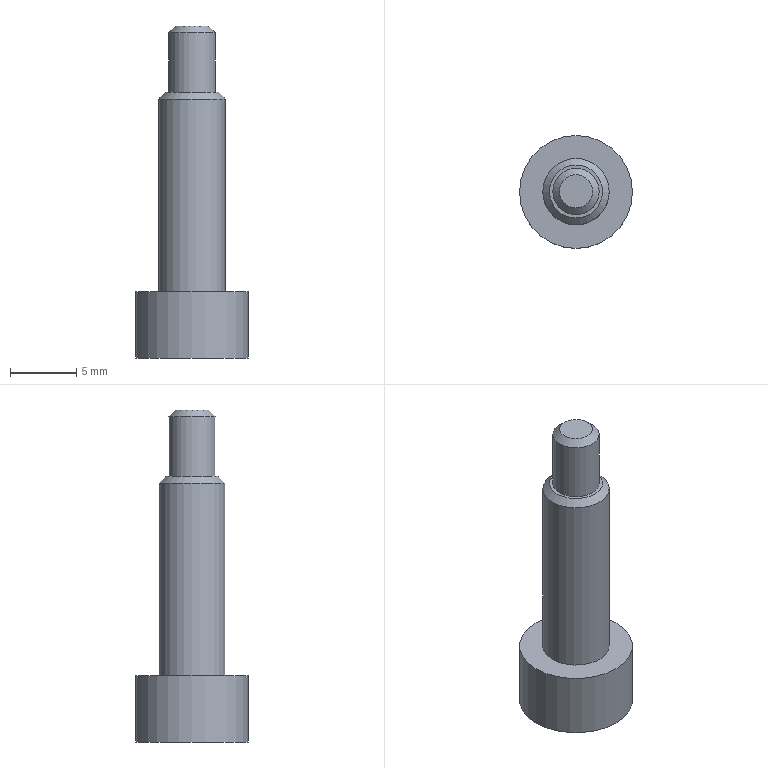Part | STEP file | 1 solid | 16 faces | box 8.5 x 8.5 x 25 mm | volume 577.553 mm3 | plane 11 | cylinder 3 | cone 2 | commonest cylinder face diameters 3.5 x1 5 x1 8.5 x1
STEP:
#1=CARTESIAN_POINT('',(0.,0.,0.));
#2=DIRECTION('',(0.,0.,1.));
#3=DIRECTION('',(1.,0.,0.));
#4=AXIS2_PLACEMENT_3D('',#1,#2,#3);
#5=CARTESIAN_POINT('',(1811.657,370.98,-34.906));
#6=VERTEX_POINT('',#5);
#7=CARTESIAN_POINT('',(1815.907,370.98,-34.906));
#8=DIRECTION('',(0.,0.,-1.));
#9=DIRECTION('',(-1.,0.,0.));
#10=AXIS2_PLACEMENT_3D('',#7,#8,#9);
#11=CIRCLE('',#10,4.25);
#12=CARTESIAN_POINT('',(1811.657,370.98,-34.906));
#13=DIRECTION('',(0.,0.,1.));
#14=DIRECTION('',(1.,0.,0.));
#15=AXIS2_PLACEMENT_3D('',#12,#13,#14);
#16=PLANE('',#15);
#17=CARTESIAN_POINT('',(0.,0.));
#18=CARTESIAN_POINT('',(0.,7.361));
#19=CARTESIAN_POINT('',(6.375,3.681));
#20=CARTESIAN_POINT('',(12.75,0.));
#21=CARTESIAN_POINT('',(6.375,-3.681));
#22=CARTESIAN_POINT('',(0.,-7.361));
#23=CARTESIAN_POINT('',(0.,0.));
#24=(BOUNDED_CURVE()B_SPLINE_CURVE(2,(#17,#18,#19,#20,#21,#22,#23),.UNSPECIFIED.,.T.,.F.)B_SPLINE_CURVE_WITH_KNOTS((1,2,2,2,2,1),(-2.094,0.,2.094,4.189,6.283,8.378),.UNSPECIFIED.)CURVE()GEOMETRIC_REPRESENTATION_ITEM()RATIONAL_B_SPLINE_CURVE((1.,0.5,1.,0.5,1.,0.5,1.))REPRESENTATION_ITEM(''));
#25=(GEOMETRIC_REPRESENTATION_CONTEXT(2)PARAMETRIC_REPRESENTATION_CONTEXT()REPRESENTATION_CONTEXT('',''));
#26=DEFINITIONAL_REPRESENTATION('',(#24),#25);
#27=PCURVE('',#16,#26);
#28=CARTESIAN_POINT('',(1815.907,370.98,1.494));
#29=DIRECTION('',(0.,0.,-1.));
#30=DIRECTION('',(-1.,0.,0.));
#31=AXIS2_PLACEMENT_3D('',#28,#29,#30);
#32=CYLINDRICAL_SURFACE('',#31,4.25);
#33=CARTESIAN_POINT('',(0.,36.4));
#34=DIRECTION('',(1.,0.));
#35=VECTOR('',#34,1.);
#36=LINE('',#33,#35);
#37=(GEOMETRIC_REPRESENTATION_CONTEXT(2)PARAMETRIC_REPRESENTATION_CONTEXT()REPRESENTATION_CONTEXT('',''));
#38=DEFINITIONAL_REPRESENTATION('',(#36),#37);
#39=PCURVE('',#32,#38);
#40=SURFACE_CURVE('',#11,(#27,#39),.PCURVE_S1.);
#41=EDGE_CURVE('',#6,#6,#40,.T.);
#42=ORIENTED_EDGE('',*,*,#41,.T.);
#43=EDGE_LOOP('',(#42));
#44=FACE_BOUND('',#43,.T.);
#45=CARTESIAN_POINT('',(1817.062,372.98,-34.906));
#46=VERTEX_POINT('',#45);
#47=CARTESIAN_POINT('',(1814.752,372.98,-34.906));
#48=VERTEX_POINT('',#47);
#49=CARTESIAN_POINT('',(1817.062,372.98,-34.906));
#50=DIRECTION('',(-1.,0.,0.));
#51=VECTOR('',#50,1.);
#52=LINE('',#49,#51);
#53=CARTESIAN_POINT('',(5.405,2.));
#54=DIRECTION('',(-1.,0.));
#55=VECTOR('',#54,1.);
#56=LINE('',#53,#55);
#57=(GEOMETRIC_REPRESENTATION_CONTEXT(2)PARAMETRIC_REPRESENTATION_CONTEXT()REPRESENTATION_CONTEXT('',''));
#58=DEFINITIONAL_REPRESENTATION('',(#56),#57);
#59=PCURVE('',#16,#58);
#60=CARTESIAN_POINT('',(1817.062,372.98,-31.606));
#61=DIRECTION('',(0.,-1.,0.));
#62=DIRECTION('',(-1.,0.,0.));
#63=AXIS2_PLACEMENT_3D('',#60,#61,#62);
#64=PLANE('',#63);
#65=CARTESIAN_POINT('',(0.,3.3));
#66=DIRECTION('',(1.,0.));
#67=VECTOR('',#66,1.);
#68=LINE('',#65,#67);
#69=(GEOMETRIC_REPRESENTATION_CONTEXT(2)PARAMETRIC_REPRESENTATION_CONTEXT()REPRESENTATION_CONTEXT('',''));
#70=DEFINITIONAL_REPRESENTATION('',(#68),#69);
#71=PCURVE('',#64,#70);
#72=SURFACE_CURVE('',#52,(#59,#71),.PCURVE_S1.);
#73=EDGE_CURVE('',#46,#48,#72,.T.);
#74=ORIENTED_EDGE('',*,*,#73,.T.);
#75=CARTESIAN_POINT('',(1813.598,370.98,-34.906));
#76=VERTEX_POINT('',#75);
#77=CARTESIAN_POINT('',(1814.752,372.98,-34.906));
#78=DIRECTION('',(-0.5,-0.866,0.));
#79=VECTOR('',#78,1.);
#80=LINE('',#77,#79);
#81=CARTESIAN_POINT('',(3.095,2.));
#82=DIRECTION('',(-0.5,-0.866));
#83=VECTOR('',#82,1.);
#84=LINE('',#81,#83);
#85=(GEOMETRIC_REPRESENTATION_CONTEXT(2)PARAMETRIC_REPRESENTATION_CONTEXT()REPRESENTATION_CONTEXT('',''));
#86=DEFINITIONAL_REPRESENTATION('',(#84),#85);
#87=PCURVE('',#16,#86);
#88=CARTESIAN_POINT('',(1814.752,372.98,-31.606));
#89=DIRECTION('',(0.866,-0.5,0.));
#90=DIRECTION('',(-0.5,-0.866,0.));
#91=AXIS2_PLACEMENT_3D('',#88,#89,#90);
#92=PLANE('',#91);
#93=CARTESIAN_POINT('',(0.,3.3));
#94=DIRECTION('',(1.,0.));
#95=VECTOR('',#94,1.);
#96=LINE('',#93,#95);
#97=(GEOMETRIC_REPRESENTATION_CONTEXT(2)PARAMETRIC_REPRESENTATION_CONTEXT()REPRESENTATION_CONTEXT('',''));
#98=DEFINITIONAL_REPRESENTATION('',(#96),#97);
#99=PCURVE('',#92,#98);
#100=SURFACE_CURVE('',#80,(#87,#99),.PCURVE_S1.);
#101=EDGE_CURVE('',#48,#76,#100,.T.);
#102=ORIENTED_EDGE('',*,*,#101,.T.);
#103=CARTESIAN_POINT('',(1814.752,368.98,-34.906));
#104=VERTEX_POINT('',#103);
#105=CARTESIAN_POINT('',(1813.598,370.98,-34.906));
#106=DIRECTION('',(0.5,-0.866,0.));
#107=VECTOR('',#106,1.);
#108=LINE('',#105,#107);
#109=CARTESIAN_POINT('',(1.941,0.));
#110=DIRECTION('',(0.5,-0.866));
#111=VECTOR('',#110,1.);
#112=LINE('',#109,#111);
#113=(GEOMETRIC_REPRESENTATION_CONTEXT(2)PARAMETRIC_REPRESENTATION_CONTEXT()REPRESENTATION_CONTEXT('',''));
#114=DEFINITIONAL_REPRESENTATION('',(#112),#113);
#115=PCURVE('',#16,#114);
#116=CARTESIAN_POINT('',(1813.598,370.98,-31.606));
#117=DIRECTION('',(0.866,0.5,0.));
#118=DIRECTION('',(0.5,-0.866,0.));
#119=AXIS2_PLACEMENT_3D('',#116,#117,#118);
#120=PLANE('',#119);
#121=CARTESIAN_POINT('',(0.,3.3));
#122=DIRECTION('',(1.,0.));
#123=VECTOR('',#122,1.);
#124=LINE('',#121,#123);
#125=(GEOMETRIC_REPRESENTATION_CONTEXT(2)PARAMETRIC_REPRESENTATION_CONTEXT()REPRESENTATION_CONTEXT('',''));
#126=DEFINITIONAL_REPRESENTATION('',(#124),#125);
#127=PCURVE('',#120,#126);
#128=SURFACE_CURVE('',#108,(#115,#127),.PCURVE_S1.);
#129=EDGE_CURVE('',#76,#104,#128,.T.);
#130=ORIENTED_EDGE('',*,*,#129,.T.);
#131=CARTESIAN_POINT('',(1817.062,368.98,-34.906));
#132=VERTEX_POINT('',#131);
#133=CARTESIAN_POINT('',(1814.752,368.98,-34.906));
#134=DIRECTION('',(1.,0.,0.));
#135=VECTOR('',#134,1.);
#136=LINE('',#133,#135);
#137=CARTESIAN_POINT('',(3.095,-2.));
#138=DIRECTION('',(1.,0.));
#139=VECTOR('',#138,1.);
#140=LINE('',#137,#139);
#141=(GEOMETRIC_REPRESENTATION_CONTEXT(2)PARAMETRIC_REPRESENTATION_CONTEXT()REPRESENTATION_CONTEXT('',''));
#142=DEFINITIONAL_REPRESENTATION('',(#140),#141);
#143=PCURVE('',#16,#142);
#144=CARTESIAN_POINT('',(1814.752,368.98,-31.606));
#145=DIRECTION('',(0.,1.,0.));
#146=DIRECTION('',(0.,0.,-1.));
#147=AXIS2_PLACEMENT_3D('',#144,#145,#146);
#148=PLANE('',#147);
#149=CARTESIAN_POINT('',(3.3,0.));
#150=DIRECTION('',(0.,-1.));
#151=VECTOR('',#150,1.);
#152=LINE('',#149,#151);
#153=(GEOMETRIC_REPRESENTATION_CONTEXT(2)PARAMETRIC_REPRESENTATION_CONTEXT()REPRESENTATION_CONTEXT('',''));
#154=DEFINITIONAL_REPRESENTATION('',(#152),#153);
#155=PCURVE('',#148,#154);
#156=SURFACE_CURVE('',#136,(#143,#155),.PCURVE_S1.);
#157=EDGE_CURVE('',#104,#132,#156,.T.);
#158=ORIENTED_EDGE('',*,*,#157,.T.);
#159=CARTESIAN_POINT('',(1818.217,370.98,-34.906));
#160=VERTEX_POINT('',#159);
#161=CARTESIAN_POINT('',(1817.062,368.98,-34.906));
#162=DIRECTION('',(0.5,0.866,0.));
#163=VECTOR('',#162,1.);
#164=LINE('',#161,#163);
#165=CARTESIAN_POINT('',(5.405,-2.));
#166=DIRECTION('',(0.5,0.866));
#167=VECTOR('',#166,1.);
#168=LINE('',#165,#167);
#169=(GEOMETRIC_REPRESENTATION_CONTEXT(2)PARAMETRIC_REPRESENTATION_CONTEXT()REPRESENTATION_CONTEXT('',''));
#170=DEFINITIONAL_REPRESENTATION('',(#168),#169);
#171=PCURVE('',#16,#170);
#172=CARTESIAN_POINT('',(1817.062,368.98,-31.606));
#173=DIRECTION('',(-0.866,0.5,0.));
#174=DIRECTION('',(0.5,0.866,0.));
#175=AXIS2_PLACEMENT_3D('',#172,#173,#174);
#176=PLANE('',#175);
#177=CARTESIAN_POINT('',(0.,3.3));
#178=DIRECTION('',(1.,0.));
#179=VECTOR('',#178,1.);
#180=LINE('',#177,#179);
#181=(GEOMETRIC_REPRESENTATION_CONTEXT(2)PARAMETRIC_REPRESENTATION_CONTEXT()REPRESENTATION_CONTEXT('',''));
#182=DEFINITIONAL_REPRESENTATION('',(#180),#181);
#183=PCURVE('',#176,#182);
#184=SURFACE_CURVE('',#164,(#171,#183),.PCURVE_S1.);
#185=EDGE_CURVE('',#132,#160,#184,.T.);
#186=ORIENTED_EDGE('',*,*,#185,.T.);
#187=CARTESIAN_POINT('',(1818.217,370.98,-34.906));
#188=DIRECTION('',(-0.5,0.866,0.));
#189=VECTOR('',#188,1.);
#190=LINE('',#187,#189);
#191=CARTESIAN_POINT('',(6.559,0.));
#192=DIRECTION('',(-0.5,0.866));
#193=VECTOR('',#192,1.);
#194=LINE('',#191,#193);
#195=(GEOMETRIC_REPRESENTATION_CONTEXT(2)PARAMETRIC_REPRESENTATION_CONTEXT()REPRESENTATION_CONTEXT('',''));
#196=DEFINITIONAL_REPRESENTATION('',(#194),#195);
#197=PCURVE('',#16,#196);
#198=CARTESIAN_POINT('',(1818.217,370.98,-31.606));
#199=DIRECTION('',(-0.866,-0.5,0.));
#200=DIRECTION('',(-0.5,0.866,0.));
#201=AXIS2_PLACEMENT_3D('',#198,#199,#200);
#202=PLANE('',#201);
#203=CARTESIAN_POINT('',(0.,3.3));
#204=DIRECTION('',(1.,0.));
#205=VECTOR('',#204,1.);
#206=LINE('',#203,#205);
#207=(GEOMETRIC_REPRESENTATION_CONTEXT(2)PARAMETRIC_REPRESENTATION_CONTEXT()REPRESENTATION_CONTEXT('',''));
#208=DEFINITIONAL_REPRESENTATION('',(#206),#207);
#209=PCURVE('',#202,#208);
#210=SURFACE_CURVE('',#190,(#197,#209),.PCURVE_S1.);
#211=EDGE_CURVE('',#160,#46,#210,.T.);
#212=ORIENTED_EDGE('',*,*,#211,.T.);
#213=EDGE_LOOP('',(#74,#102,#130,#158,#186,#212));
#214=FACE_BOUND('',#213,.T.);
#215=ADVANCED_FACE('',(#44,#214),#16,.F.);
#216=ORIENTED_EDGE('',*,*,#41,.F.);
#217=CARTESIAN_POINT('',(1811.657,370.98,-29.906));
#218=VERTEX_POINT('',#217);
#219=CARTESIAN_POINT('',(1811.657,370.98,-29.906));
#220=CARTESIAN_POINT('',(1811.657,370.98,-34.906));
#221=B_SPLINE_CURVE_WITH_KNOTS('',1,(#219,#220),.UNSPECIFIED.,.F.,.F.,(2,2),(31.4,36.4),.PIECEWISE_BEZIER_KNOTS.);
#222=CARTESIAN_POINT('',(0.,0.));
#223=DIRECTION('',(0.,1.));
#224=VECTOR('',#223,1.);
#225=LINE('',#222,#224);
#226=(GEOMETRIC_REPRESENTATION_CONTEXT(2)PARAMETRIC_REPRESENTATION_CONTEXT()REPRESENTATION_CONTEXT('',''));
#227=DEFINITIONAL_REPRESENTATION('',(#225),#226);
#228=PCURVE('',#32,#227);
#229=CARTESIAN_POINT('',(6.283,0.));
#230=DIRECTION('',(0.,1.));
#231=VECTOR('',#230,1.);
#232=LINE('',#229,#231);
#233=(GEOMETRIC_REPRESENTATION_CONTEXT(2)PARAMETRIC_REPRESENTATION_CONTEXT()REPRESENTATION_CONTEXT('',''));
#234=DEFINITIONAL_REPRESENTATION('',(#232),#233);
#235=PCURVE('',#32,#234);
#236=SEAM_CURVE('',#221,(#228,#235),.PCURVE_S1.);
#237=EDGE_CURVE('',#218,#6,#236,.T.);
#238=ORIENTED_EDGE('',*,*,#237,.F.);
#239=CARTESIAN_POINT('',(1815.907,370.98,-29.906));
#240=DIRECTION('',(0.,0.,-1.));
#241=DIRECTION('',(-1.,0.,0.));
#242=AXIS2_PLACEMENT_3D('',#239,#240,#241);
#243=CIRCLE('',#242,4.25);
#244=CARTESIAN_POINT('',(0.,31.4));
#245=DIRECTION('',(1.,0.));
#246=VECTOR('',#245,1.);
#247=LINE('',#244,#246);
#248=(GEOMETRIC_REPRESENTATION_CONTEXT(2)PARAMETRIC_REPRESENTATION_CONTEXT()REPRESENTATION_CONTEXT('',''));
#249=DEFINITIONAL_REPRESENTATION('',(#247),#248);
#250=PCURVE('',#32,#249);
#251=CARTESIAN_POINT('',(1813.407,370.98,-29.906));
#252=DIRECTION('',(0.,0.,-1.));
#253=DIRECTION('',(-1.,0.,0.));
#254=AXIS2_PLACEMENT_3D('',#251,#252,#253);
#255=PLANE('',#254);
#256=CARTESIAN_POINT('',(-2.5,0.));
#257=DIRECTION('',(1.,0.));
#258=AXIS2_PLACEMENT_2D('',#256,#257);
#259=CIRCLE('',#258,4.25);
#260=(GEOMETRIC_REPRESENTATION_CONTEXT(2)PARAMETRIC_REPRESENTATION_CONTEXT()REPRESENTATION_CONTEXT('',''));
#261=DEFINITIONAL_REPRESENTATION('',(#259),#260);
#262=PCURVE('',#255,#261);
#263=SURFACE_CURVE('',#243,(#250,#262),.PCURVE_S1.);
#264=EDGE_CURVE('',#218,#218,#263,.T.);
#265=ORIENTED_EDGE('',*,*,#264,.T.);
#266=ORIENTED_EDGE('',*,*,#237,.T.);
#267=EDGE_LOOP('',(#216,#238,#265,#266));
#268=FACE_BOUND('',#267,.T.);
#269=ADVANCED_FACE('',(#268),#32,.T.);
#270=ORIENTED_EDGE('',*,*,#264,.F.);
#271=EDGE_LOOP('',(#270));
#272=FACE_BOUND('',#271,.T.);
#273=CARTESIAN_POINT('',(1813.407,370.98,-29.906));
#274=VERTEX_POINT('',#273);
#275=CARTESIAN_POINT('',(1815.907,370.98,-29.906));
#276=DIRECTION('',(0.,0.,-1.));
#277=DIRECTION('',(-1.,0.,0.));
#278=AXIS2_PLACEMENT_3D('',#275,#276,#277);
#279=CIRCLE('',#278,2.5);
#280=CARTESIAN_POINT('',(-2.5,0.));
#281=DIRECTION('',(1.,0.));
#282=AXIS2_PLACEMENT_2D('',#280,#281);
#283=CIRCLE('',#282,2.5);
#284=(GEOMETRIC_REPRESENTATION_CONTEXT(2)PARAMETRIC_REPRESENTATION_CONTEXT()REPRESENTATION_CONTEXT('',''));
#285=DEFINITIONAL_REPRESENTATION('',(#283),#284);
#286=PCURVE('',#255,#285);
#287=CARTESIAN_POINT('',(1815.907,370.98,1.494));
#288=DIRECTION('',(0.,0.,-1.));
#289=DIRECTION('',(-1.,0.,0.));
#290=AXIS2_PLACEMENT_3D('',#287,#288,#289);
#291=CYLINDRICAL_SURFACE('',#290,2.5);
#292=CARTESIAN_POINT('',(0.,31.4));
#293=DIRECTION('',(1.,0.));
#294=VECTOR('',#293,1.);
#295=LINE('',#292,#294);
#296=(GEOMETRIC_REPRESENTATION_CONTEXT(2)PARAMETRIC_REPRESENTATION_CONTEXT()REPRESENTATION_CONTEXT('',''));
#297=DEFINITIONAL_REPRESENTATION('',(#295),#296);
#298=PCURVE('',#291,#297);
#299=SURFACE_CURVE('',#279,(#286,#298),.PCURVE_S1.);
#300=EDGE_CURVE('',#274,#274,#299,.T.);
#301=ORIENTED_EDGE('',*,*,#300,.T.);
#302=EDGE_LOOP('',(#301));
#303=FACE_BOUND('',#302,.T.);
#304=ADVANCED_FACE('',(#272,#303),#255,.F.);
#305=CARTESIAN_POINT('',(1818.407,370.98,-15.406));
#306=VERTEX_POINT('',#305);
#307=CARTESIAN_POINT('',(1813.407,370.98,-15.406));
#308=VERTEX_POINT('',#307);
#309=CARTESIAN_POINT('',(1815.907,370.98,-15.406));
#310=DIRECTION('',(0.,0.,-1.));
#311=DIRECTION('',(1.,0.,0.));
#312=AXIS2_PLACEMENT_3D('',#309,#310,#311);
#313=CIRCLE('',#312,2.5);
#314=CARTESIAN_POINT('',(3.142,16.9));
#315=DIRECTION('',(1.,0.));
#316=VECTOR('',#315,1.);
#317=LINE('',#314,#316);
#318=(GEOMETRIC_REPRESENTATION_CONTEXT(2)PARAMETRIC_REPRESENTATION_CONTEXT()REPRESENTATION_CONTEXT('',''));
#319=DEFINITIONAL_REPRESENTATION('',(#317),#318);
#320=PCURVE('',#291,#319);
#321=CARTESIAN_POINT('',(1815.907,370.98,-15.406));
#322=DIRECTION('',(0.,0.,-1.));
#323=DIRECTION('',(-1.,0.,0.));
#324=AXIS2_PLACEMENT_3D('',#321,#322,#323);
#325=CONICAL_SURFACE('',#324,2.5,0.7854);
#326=CARTESIAN_POINT('',(3.142,0.));
#327=DIRECTION('',(1.,0.));
#328=VECTOR('',#327,1.);
#329=LINE('',#326,#328);
#330=(GEOMETRIC_REPRESENTATION_CONTEXT(2)PARAMETRIC_REPRESENTATION_CONTEXT()REPRESENTATION_CONTEXT('',''));
#331=DEFINITIONAL_REPRESENTATION('',(#329),#330);
#332=PCURVE('',#325,#331);
#333=SURFACE_CURVE('',#313,(#320,#332),.PCURVE_S1.);
#334=EDGE_CURVE('',#306,#308,#333,.T.);
#335=ORIENTED_EDGE('',*,*,#334,.T.);
#336=CARTESIAN_POINT('',(1813.407,370.98,-15.406));
#337=CARTESIAN_POINT('',(1813.407,370.98,-29.906));
#338=B_SPLINE_CURVE_WITH_KNOTS('',1,(#336,#337),.UNSPECIFIED.,.F.,.F.,(2,2),(16.9,31.4),.PIECEWISE_BEZIER_KNOTS.);
#339=CARTESIAN_POINT('',(6.283,0.));
#340=DIRECTION('',(0.,1.));
#341=VECTOR('',#340,1.);
#342=LINE('',#339,#341);
#343=(GEOMETRIC_REPRESENTATION_CONTEXT(2)PARAMETRIC_REPRESENTATION_CONTEXT()REPRESENTATION_CONTEXT('',''));
#344=DEFINITIONAL_REPRESENTATION('',(#342),#343);
#345=PCURVE('',#291,#344);
#346=CARTESIAN_POINT('',(0.,0.));
#347=DIRECTION('',(0.,1.));
#348=VECTOR('',#347,1.);
#349=LINE('',#346,#348);
#350=(GEOMETRIC_REPRESENTATION_CONTEXT(2)PARAMETRIC_REPRESENTATION_CONTEXT()REPRESENTATION_CONTEXT('',''));
#351=DEFINITIONAL_REPRESENTATION('',(#349),#350);
#352=PCURVE('',#291,#351);
#353=SEAM_CURVE('',#338,(#345,#352),.PCURVE_S1.);
#354=EDGE_CURVE('',#308,#274,#353,.T.);
#355=ORIENTED_EDGE('',*,*,#354,.T.);
#356=ORIENTED_EDGE('',*,*,#300,.F.);
#357=ORIENTED_EDGE('',*,*,#354,.F.);
#358=CARTESIAN_POINT('',(1815.907,370.98,-15.406));
#359=DIRECTION('',(0.,0.,-1.));
#360=DIRECTION('',(1.,0.,0.));
#361=AXIS2_PLACEMENT_3D('',#358,#359,#360);
#362=CIRCLE('',#361,2.5);
#363=CARTESIAN_POINT('',(-3.142,16.9));
#364=DIRECTION('',(1.,0.));
#365=VECTOR('',#364,1.);
#366=LINE('',#363,#365);
#367=(GEOMETRIC_REPRESENTATION_CONTEXT(2)PARAMETRIC_REPRESENTATION_CONTEXT()REPRESENTATION_CONTEXT('',''));
#368=DEFINITIONAL_REPRESENTATION('',(#366),#367);
#369=PCURVE('',#291,#368);
#370=CARTESIAN_POINT('',(3.142,0.));
#371=DIRECTION('',(1.,0.));
#372=VECTOR('',#371,1.);
#373=LINE('',#370,#372);
#374=(GEOMETRIC_REPRESENTATION_CONTEXT(2)PARAMETRIC_REPRESENTATION_CONTEXT()REPRESENTATION_CONTEXT('',''));
#375=DEFINITIONAL_REPRESENTATION('',(#373),#374);
#376=PCURVE('',#325,#375);
#377=SURFACE_CURVE('',#362,(#369,#376),.PCURVE_S1.);
#378=EDGE_CURVE('',#308,#306,#377,.T.);
#379=ORIENTED_EDGE('',*,*,#378,.T.);
#380=EDGE_LOOP('',(#335,#355,#356,#357,#379));
#381=FACE_BOUND('',#380,.T.);
#382=ADVANCED_FACE('',(#381),#291,.T.);
#383=ORIENTED_EDGE('',*,*,#73,.F.);
#384=CARTESIAN_POINT('',(1817.062,372.98,-31.606));
#385=VERTEX_POINT('',#384);
#386=CARTESIAN_POINT('',(1817.062,372.98,-31.606));
#387=DIRECTION('',(0.,0.,1.));
#388=VECTOR('',#387,1.);
#389=LINE('',#386,#388);
#390=CARTESIAN_POINT('',(0.,0.));
#391=DIRECTION('',(0.,-1.));
#392=VECTOR('',#391,1.);
#393=LINE('',#390,#392);
#394=(GEOMETRIC_REPRESENTATION_CONTEXT(2)PARAMETRIC_REPRESENTATION_CONTEXT()REPRESENTATION_CONTEXT('',''));
#395=DEFINITIONAL_REPRESENTATION('',(#393),#394);
#396=PCURVE('',#64,#395);
#397=CARTESIAN_POINT('',(2.309,0.));
#398=DIRECTION('',(0.,-1.));
#399=VECTOR('',#398,1.);
#400=LINE('',#397,#399);
#401=(GEOMETRIC_REPRESENTATION_CONTEXT(2)PARAMETRIC_REPRESENTATION_CONTEXT()REPRESENTATION_CONTEXT('',''));
#402=DEFINITIONAL_REPRESENTATION('',(#400),#401);
#403=PCURVE('',#202,#402);
#404=SURFACE_CURVE('',#389,(#396,#403),.PCURVE_S1.);
#405=EDGE_CURVE('',#46,#385,#404,.T.);
#406=ORIENTED_EDGE('',*,*,#405,.T.);
#407=CARTESIAN_POINT('',(1814.752,372.98,-31.606));
#408=VERTEX_POINT('',#407);
#409=CARTESIAN_POINT('',(1817.062,372.98,-31.606));
#410=DIRECTION('',(1.,0.,0.));
#411=VECTOR('',#410,1.);
#412=LINE('',#409,#411);
#413=CARTESIAN_POINT('',(0.,0.));
#414=DIRECTION('',(-1.,0.));
#415=VECTOR('',#414,1.);
#416=LINE('',#413,#415);
#417=(GEOMETRIC_REPRESENTATION_CONTEXT(2)PARAMETRIC_REPRESENTATION_CONTEXT()REPRESENTATION_CONTEXT('',''));
#418=DEFINITIONAL_REPRESENTATION('',(#416),#417);
#419=PCURVE('',#64,#418);
#420=CARTESIAN_POINT('',(1815.907,370.98,-31.606));
#421=DIRECTION('',(0.,0.,1.));
#422=DIRECTION('',(1.,0.,0.));
#423=AXIS2_PLACEMENT_3D('',#420,#421,#422);
#424=PLANE('',#423);
#425=CARTESIAN_POINT('',(1.155,2.));
#426=DIRECTION('',(1.,0.));
#427=VECTOR('',#426,1.);
#428=LINE('',#425,#427);
#429=(GEOMETRIC_REPRESENTATION_CONTEXT(2)PARAMETRIC_REPRESENTATION_CONTEXT()REPRESENTATION_CONTEXT('',''));
#430=DEFINITIONAL_REPRESENTATION('',(#428),#429);
#431=PCURVE('',#424,#430);
#432=SURFACE_CURVE('',#412,(#419,#431),.PCURVE_S1.);
#433=EDGE_CURVE('',#408,#385,#432,.T.);
#434=ORIENTED_EDGE('',*,*,#433,.F.);
#435=CARTESIAN_POINT('',(1814.752,372.98,-31.606));
#436=DIRECTION('',(0.,0.,1.));
#437=VECTOR('',#436,1.);
#438=LINE('',#435,#437);
#439=CARTESIAN_POINT('',(2.309,0.));
#440=DIRECTION('',(0.,-1.));
#441=VECTOR('',#440,1.);
#442=LINE('',#439,#441);
#443=(GEOMETRIC_REPRESENTATION_CONTEXT(2)PARAMETRIC_REPRESENTATION_CONTEXT()REPRESENTATION_CONTEXT('',''));
#444=DEFINITIONAL_REPRESENTATION('',(#442),#443);
#445=PCURVE('',#64,#444);
#446=CARTESIAN_POINT('',(0.,0.));
#447=DIRECTION('',(0.,-1.));
#448=VECTOR('',#447,1.);
#449=LINE('',#446,#448);
#450=(GEOMETRIC_REPRESENTATION_CONTEXT(2)PARAMETRIC_REPRESENTATION_CONTEXT()REPRESENTATION_CONTEXT('',''));
#451=DEFINITIONAL_REPRESENTATION('',(#449),#450);
#452=PCURVE('',#92,#451);
#453=SURFACE_CURVE('',#438,(#445,#452),.PCURVE_S1.);
#454=EDGE_CURVE('',#48,#408,#453,.T.);
#455=ORIENTED_EDGE('',*,*,#454,.F.);
#456=EDGE_LOOP('',(#383,#406,#434,#455));
#457=FACE_BOUND('',#456,.T.);
#458=ADVANCED_FACE('',(#457),#64,.T.);
#459=ORIENTED_EDGE('',*,*,#101,.F.);
#460=ORIENTED_EDGE('',*,*,#454,.T.);
#461=CARTESIAN_POINT('',(1813.598,370.98,-31.606));
#462=VERTEX_POINT('',#461);
#463=CARTESIAN_POINT('',(1814.752,372.98,-31.606));
#464=DIRECTION('',(0.5,0.866,0.));
#465=VECTOR('',#464,1.);
#466=LINE('',#463,#465);
#467=CARTESIAN_POINT('',(0.,0.));
#468=DIRECTION('',(-1.,0.));
#469=VECTOR('',#468,1.);
#470=LINE('',#467,#469);
#471=(GEOMETRIC_REPRESENTATION_CONTEXT(2)PARAMETRIC_REPRESENTATION_CONTEXT()REPRESENTATION_CONTEXT('',''));
#472=DEFINITIONAL_REPRESENTATION('',(#470),#471);
#473=PCURVE('',#92,#472);
#474=CARTESIAN_POINT('',(-1.155,2.));
#475=DIRECTION('',(0.5,0.866));
#476=VECTOR('',#475,1.);
#477=LINE('',#474,#476);
#478=(GEOMETRIC_REPRESENTATION_CONTEXT(2)PARAMETRIC_REPRESENTATION_CONTEXT()REPRESENTATION_CONTEXT('',''));
#479=DEFINITIONAL_REPRESENTATION('',(#477),#478);
#480=PCURVE('',#424,#479);
#481=SURFACE_CURVE('',#466,(#473,#480),.PCURVE_S1.);
#482=EDGE_CURVE('',#462,#408,#481,.T.);
#483=ORIENTED_EDGE('',*,*,#482,.F.);
#484=CARTESIAN_POINT('',(1813.598,370.98,-31.606));
#485=DIRECTION('',(0.,0.,1.));
#486=VECTOR('',#485,1.);
#487=LINE('',#484,#486);
#488=CARTESIAN_POINT('',(2.309,0.));
#489=DIRECTION('',(0.,-1.));
#490=VECTOR('',#489,1.);
#491=LINE('',#488,#490);
#492=(GEOMETRIC_REPRESENTATION_CONTEXT(2)PARAMETRIC_REPRESENTATION_CONTEXT()REPRESENTATION_CONTEXT('',''));
#493=DEFINITIONAL_REPRESENTATION('',(#491),#492);
#494=PCURVE('',#92,#493);
#495=CARTESIAN_POINT('',(0.,0.));
#496=DIRECTION('',(0.,-1.));
#497=VECTOR('',#496,1.);
#498=LINE('',#495,#497);
#499=(GEOMETRIC_REPRESENTATION_CONTEXT(2)PARAMETRIC_REPRESENTATION_CONTEXT()REPRESENTATION_CONTEXT('',''));
#500=DEFINITIONAL_REPRESENTATION('',(#498),#499);
#501=PCURVE('',#120,#500);
#502=SURFACE_CURVE('',#487,(#494,#501),.PCURVE_S1.);
#503=EDGE_CURVE('',#76,#462,#502,.T.);
#504=ORIENTED_EDGE('',*,*,#503,.F.);
#505=EDGE_LOOP('',(#459,#460,#483,#504));
#506=FACE_BOUND('',#505,.T.);
#507=ADVANCED_FACE('',(#506),#92,.T.);
#508=ORIENTED_EDGE('',*,*,#129,.F.);
#509=ORIENTED_EDGE('',*,*,#503,.T.);
#510=CARTESIAN_POINT('',(1814.752,368.98,-31.606));
#511=VERTEX_POINT('',#510);
#512=CARTESIAN_POINT('',(1813.598,370.98,-31.606));
#513=DIRECTION('',(-0.5,0.866,0.));
#514=VECTOR('',#513,1.);
#515=LINE('',#512,#514);
#516=CARTESIAN_POINT('',(0.,0.));
#517=DIRECTION('',(-1.,0.));
#518=VECTOR('',#517,1.);
#519=LINE('',#516,#518);
#520=(GEOMETRIC_REPRESENTATION_CONTEXT(2)PARAMETRIC_REPRESENTATION_CONTEXT()REPRESENTATION_CONTEXT('',''));
#521=DEFINITIONAL_REPRESENTATION('',(#519),#520);
#522=PCURVE('',#120,#521);
#523=CARTESIAN_POINT('',(-2.309,0.));
#524=DIRECTION('',(-0.5,0.866));
#525=VECTOR('',#524,1.);
#526=LINE('',#523,#525);
#527=(GEOMETRIC_REPRESENTATION_CONTEXT(2)PARAMETRIC_REPRESENTATION_CONTEXT()REPRESENTATION_CONTEXT('',''));
#528=DEFINITIONAL_REPRESENTATION('',(#526),#527);
#529=PCURVE('',#424,#528);
#530=SURFACE_CURVE('',#515,(#522,#529),.PCURVE_S1.);
#531=EDGE_CURVE('',#511,#462,#530,.T.);
#532=ORIENTED_EDGE('',*,*,#531,.F.);
#533=CARTESIAN_POINT('',(1814.752,368.98,-31.606));
#534=DIRECTION('',(0.,0.,1.));
#535=VECTOR('',#534,1.);
#536=LINE('',#533,#535);
#537=CARTESIAN_POINT('',(2.309,0.));
#538=DIRECTION('',(0.,-1.));
#539=VECTOR('',#538,1.);
#540=LINE('',#537,#539);
#541=(GEOMETRIC_REPRESENTATION_CONTEXT(2)PARAMETRIC_REPRESENTATION_CONTEXT()REPRESENTATION_CONTEXT('',''));
#542=DEFINITIONAL_REPRESENTATION('',(#540),#541);
#543=PCURVE('',#120,#542);
#544=CARTESIAN_POINT('',(0.,0.));
#545=DIRECTION('',(-1.,0.));
#546=VECTOR('',#545,1.);
#547=LINE('',#544,#546);
#548=(GEOMETRIC_REPRESENTATION_CONTEXT(2)PARAMETRIC_REPRESENTATION_CONTEXT()REPRESENTATION_CONTEXT('',''));
#549=DEFINITIONAL_REPRESENTATION('',(#547),#548);
#550=PCURVE('',#148,#549);
#551=SURFACE_CURVE('',#536,(#543,#550),.PCURVE_S1.);
#552=EDGE_CURVE('',#104,#511,#551,.T.);
#553=ORIENTED_EDGE('',*,*,#552,.F.);
#554=EDGE_LOOP('',(#508,#509,#532,#553));
#555=FACE_BOUND('',#554,.T.);
#556=ADVANCED_FACE('',(#555),#120,.T.);
#557=ORIENTED_EDGE('',*,*,#157,.F.);
#558=ORIENTED_EDGE('',*,*,#552,.T.);
#559=CARTESIAN_POINT('',(1817.062,368.98,-31.606));
#560=VERTEX_POINT('',#559);
#561=CARTESIAN_POINT('',(1814.752,368.98,-31.606));
#562=DIRECTION('',(-1.,0.,0.));
#563=VECTOR('',#562,1.);
#564=LINE('',#561,#563);
#565=CARTESIAN_POINT('',(0.,0.));
#566=DIRECTION('',(0.,1.));
#567=VECTOR('',#566,1.);
#568=LINE('',#565,#567);
#569=(GEOMETRIC_REPRESENTATION_CONTEXT(2)PARAMETRIC_REPRESENTATION_CONTEXT()REPRESENTATION_CONTEXT('',''));
#570=DEFINITIONAL_REPRESENTATION('',(#568),#569);
#571=PCURVE('',#148,#570);
#572=CARTESIAN_POINT('',(-1.155,-2.));
#573=DIRECTION('',(-1.,0.));
#574=VECTOR('',#573,1.);
#575=LINE('',#572,#574);
#576=(GEOMETRIC_REPRESENTATION_CONTEXT(2)PARAMETRIC_REPRESENTATION_CONTEXT()REPRESENTATION_CONTEXT('',''));
#577=DEFINITIONAL_REPRESENTATION('',(#575),#576);
#578=PCURVE('',#424,#577);
#579=SURFACE_CURVE('',#564,(#571,#578),.PCURVE_S1.);
#580=EDGE_CURVE('',#560,#511,#579,.T.);
#581=ORIENTED_EDGE('',*,*,#580,.F.);
#582=CARTESIAN_POINT('',(1817.062,368.98,-31.606));
#583=DIRECTION('',(0.,0.,1.));
#584=VECTOR('',#583,1.);
#585=LINE('',#582,#584);
#586=CARTESIAN_POINT('',(0.,-2.309));
#587=DIRECTION('',(-1.,0.));
#588=VECTOR('',#587,1.);
#589=LINE('',#586,#588);
#590=(GEOMETRIC_REPRESENTATION_CONTEXT(2)PARAMETRIC_REPRESENTATION_CONTEXT()REPRESENTATION_CONTEXT('',''));
#591=DEFINITIONAL_REPRESENTATION('',(#589),#590);
#592=PCURVE('',#148,#591);
#593=CARTESIAN_POINT('',(0.,0.));
#594=DIRECTION('',(0.,-1.));
#595=VECTOR('',#594,1.);
#596=LINE('',#593,#595);
#597=(GEOMETRIC_REPRESENTATION_CONTEXT(2)PARAMETRIC_REPRESENTATION_CONTEXT()REPRESENTATION_CONTEXT('',''));
#598=DEFINITIONAL_REPRESENTATION('',(#596),#597);
#599=PCURVE('',#176,#598);
#600=SURFACE_CURVE('',#585,(#592,#599),.PCURVE_S1.);
#601=EDGE_CURVE('',#132,#560,#600,.T.);
#602=ORIENTED_EDGE('',*,*,#601,.F.);
#603=EDGE_LOOP('',(#557,#558,#581,#602));
#604=FACE_BOUND('',#603,.T.);
#605=ADVANCED_FACE('',(#604),#148,.T.);
#606=ORIENTED_EDGE('',*,*,#185,.F.);
#607=ORIENTED_EDGE('',*,*,#601,.T.);
#608=CARTESIAN_POINT('',(1818.217,370.98,-31.606));
#609=VERTEX_POINT('',#608);
#610=CARTESIAN_POINT('',(1817.062,368.98,-31.606));
#611=DIRECTION('',(-0.5,-0.866,0.));
#612=VECTOR('',#611,1.);
#613=LINE('',#610,#612);
#614=CARTESIAN_POINT('',(0.,0.));
#615=DIRECTION('',(-1.,0.));
#616=VECTOR('',#615,1.);
#617=LINE('',#614,#616);
#618=(GEOMETRIC_REPRESENTATION_CONTEXT(2)PARAMETRIC_REPRESENTATION_CONTEXT()REPRESENTATION_CONTEXT('',''));
#619=DEFINITIONAL_REPRESENTATION('',(#617),#618);
#620=PCURVE('',#176,#619);
#621=CARTESIAN_POINT('',(1.155,-2.));
#622=DIRECTION('',(-0.5,-0.866));
#623=VECTOR('',#622,1.);
#624=LINE('',#621,#623);
#625=(GEOMETRIC_REPRESENTATION_CONTEXT(2)PARAMETRIC_REPRESENTATION_CONTEXT()REPRESENTATION_CONTEXT('',''));
#626=DEFINITIONAL_REPRESENTATION('',(#624),#625);
#627=PCURVE('',#424,#626);
#628=SURFACE_CURVE('',#613,(#620,#627),.PCURVE_S1.);
#629=EDGE_CURVE('',#609,#560,#628,.T.);
#630=ORIENTED_EDGE('',*,*,#629,.F.);
#631=CARTESIAN_POINT('',(1818.217,370.98,-31.606));
#632=DIRECTION('',(0.,0.,1.));
#633=VECTOR('',#632,1.);
#634=LINE('',#631,#633);
#635=CARTESIAN_POINT('',(2.309,0.));
#636=DIRECTION('',(0.,-1.));
#637=VECTOR('',#636,1.);
#638=LINE('',#635,#637);
#639=(GEOMETRIC_REPRESENTATION_CONTEXT(2)PARAMETRIC_REPRESENTATION_CONTEXT()REPRESENTATION_CONTEXT('',''));
#640=DEFINITIONAL_REPRESENTATION('',(#638),#639);
#641=PCURVE('',#176,#640);
#642=CARTESIAN_POINT('',(0.,0.));
#643=DIRECTION('',(0.,-1.));
#644=VECTOR('',#643,1.);
#645=LINE('',#642,#644);
#646=(GEOMETRIC_REPRESENTATION_CONTEXT(2)PARAMETRIC_REPRESENTATION_CONTEXT()REPRESENTATION_CONTEXT('',''));
#647=DEFINITIONAL_REPRESENTATION('',(#645),#646);
#648=PCURVE('',#202,#647);
#649=SURFACE_CURVE('',#634,(#641,#648),.PCURVE_S1.);
#650=EDGE_CURVE('',#160,#609,#649,.T.);
#651=ORIENTED_EDGE('',*,*,#650,.F.);
#652=EDGE_LOOP('',(#606,#607,#630,#651));
#653=FACE_BOUND('',#652,.T.);
#654=ADVANCED_FACE('',(#653),#176,.T.);
#655=ORIENTED_EDGE('',*,*,#211,.F.);
#656=ORIENTED_EDGE('',*,*,#650,.T.);
#657=CARTESIAN_POINT('',(1818.217,370.98,-31.606));
#658=DIRECTION('',(0.5,-0.866,0.));
#659=VECTOR('',#658,1.);
#660=LINE('',#657,#659);
#661=CARTESIAN_POINT('',(0.,0.));
#662=DIRECTION('',(-1.,0.));
#663=VECTOR('',#662,1.);
#664=LINE('',#661,#663);
#665=(GEOMETRIC_REPRESENTATION_CONTEXT(2)PARAMETRIC_REPRESENTATION_CONTEXT()REPRESENTATION_CONTEXT('',''));
#666=DEFINITIONAL_REPRESENTATION('',(#664),#665);
#667=PCURVE('',#202,#666);
#668=CARTESIAN_POINT('',(2.309,0.));
#669=DIRECTION('',(0.5,-0.866));
#670=VECTOR('',#669,1.);
#671=LINE('',#668,#670);
#672=(GEOMETRIC_REPRESENTATION_CONTEXT(2)PARAMETRIC_REPRESENTATION_CONTEXT()REPRESENTATION_CONTEXT('',''));
#673=DEFINITIONAL_REPRESENTATION('',(#671),#672);
#674=PCURVE('',#424,#673);
#675=SURFACE_CURVE('',#660,(#667,#674),.PCURVE_S1.);
#676=EDGE_CURVE('',#385,#609,#675,.T.);
#677=ORIENTED_EDGE('',*,*,#676,.F.);
#678=ORIENTED_EDGE('',*,*,#405,.F.);
#679=EDGE_LOOP('',(#655,#656,#677,#678));
#680=FACE_BOUND('',#679,.T.);
#681=ADVANCED_FACE('',(#680),#202,.T.);
#682=ORIENTED_EDGE('',*,*,#433,.T.);
#683=ORIENTED_EDGE('',*,*,#676,.T.);
#684=ORIENTED_EDGE('',*,*,#629,.T.);
#685=ORIENTED_EDGE('',*,*,#580,.T.);
#686=ORIENTED_EDGE('',*,*,#531,.T.);
#687=ORIENTED_EDGE('',*,*,#482,.T.);
#688=EDGE_LOOP('',(#682,#683,#684,#685,#686,#687));
#689=FACE_BOUND('',#688,.T.);
#690=ADVANCED_FACE('',(#689),#424,.F.);
#691=CARTESIAN_POINT('',(1817.907,370.98,-14.906));
#692=VERTEX_POINT('',#691);
#693=CARTESIAN_POINT('',(1815.907,370.98,-14.906));
#694=DIRECTION('',(0.,0.,1.));
#695=DIRECTION('',(1.,0.,0.));
#696=AXIS2_PLACEMENT_3D('',#693,#694,#695);
#697=CIRCLE('',#696,2.);
#698=CARTESIAN_POINT('',(1815.907,370.98,-14.906));
#699=DIRECTION('',(0.,0.,1.));
#700=DIRECTION('',(1.,0.,0.));
#701=AXIS2_PLACEMENT_3D('',#698,#699,#700);
#702=PLANE('',#701);
#703=CARTESIAN_POINT('',(0.,0.));
#704=DIRECTION('',(1.,0.));
#705=AXIS2_PLACEMENT_2D('',#703,#704);
#706=CIRCLE('',#705,2.);
#707=(GEOMETRIC_REPRESENTATION_CONTEXT(2)PARAMETRIC_REPRESENTATION_CONTEXT()REPRESENTATION_CONTEXT('',''));
#708=DEFINITIONAL_REPRESENTATION('',(#706),#707);
#709=PCURVE('',#702,#708);
#710=CARTESIAN_POINT('',(9.425,-0.5));
#711=DIRECTION('',(-1.,0.));
#712=VECTOR('',#711,1.);
#713=LINE('',#710,#712);
#714=(GEOMETRIC_REPRESENTATION_CONTEXT(2)PARAMETRIC_REPRESENTATION_CONTEXT()REPRESENTATION_CONTEXT('',''));
#715=DEFINITIONAL_REPRESENTATION('',(#713),#714);
#716=PCURVE('',#325,#715);
#717=SURFACE_CURVE('',#697,(#709,#716),.PCURVE_S1.);
#718=EDGE_CURVE('',#692,#692,#717,.T.);
#719=ORIENTED_EDGE('',*,*,#718,.T.);
#720=EDGE_LOOP('',(#719));
#721=FACE_BOUND('',#720,.T.);
#722=CARTESIAN_POINT('',(1817.657,370.98,-14.906));
#723=VERTEX_POINT('',#722);
#724=CARTESIAN_POINT('',(1814.157,370.98,-14.906));
#725=VERTEX_POINT('',#724);
#726=CARTESIAN_POINT('',(1815.907,370.98,-14.906));
#727=DIRECTION('',(0.,0.,1.));
#728=DIRECTION('',(1.,0.,0.));
#729=AXIS2_PLACEMENT_3D('',#726,#727,#728);
#730=CIRCLE('',#729,1.75);
#731=CARTESIAN_POINT('',(0.,0.));
#732=DIRECTION('',(1.,0.));
#733=AXIS2_PLACEMENT_2D('',#731,#732);
#734=CIRCLE('',#733,1.75);
#735=(GEOMETRIC_REPRESENTATION_CONTEXT(2)PARAMETRIC_REPRESENTATION_CONTEXT()REPRESENTATION_CONTEXT('',''));
#736=DEFINITIONAL_REPRESENTATION('',(#734),#735);
#737=PCURVE('',#702,#736);
#738=CARTESIAN_POINT('',(1815.907,370.98,-9.906));
#739=DIRECTION('',(0.,0.,-1.));
#740=DIRECTION('',(-1.,0.,0.));
#741=AXIS2_PLACEMENT_3D('',#738,#739,#740);
#742=CYLINDRICAL_SURFACE('',#741,1.75);
#743=CARTESIAN_POINT('',(3.142,5.));
#744=DIRECTION('',(-1.,0.));
#745=VECTOR('',#744,1.);
#746=LINE('',#743,#745);
#747=(GEOMETRIC_REPRESENTATION_CONTEXT(2)PARAMETRIC_REPRESENTATION_CONTEXT()REPRESENTATION_CONTEXT('',''));
#748=DEFINITIONAL_REPRESENTATION('',(#746),#747);
#749=PCURVE('',#742,#748);
#750=SURFACE_CURVE('',#730,(#737,#749),.PCURVE_S1.);
#751=EDGE_CURVE('',#723,#725,#750,.T.);
#752=ORIENTED_EDGE('',*,*,#751,.F.);
#753=CARTESIAN_POINT('',(1815.907,370.98,-14.906));
#754=DIRECTION('',(0.,0.,1.));
#755=DIRECTION('',(1.,0.,0.));
#756=AXIS2_PLACEMENT_3D('',#753,#754,#755);
#757=CIRCLE('',#756,1.75);
#758=CARTESIAN_POINT('',(0.,0.));
#759=DIRECTION('',(1.,0.));
#760=AXIS2_PLACEMENT_2D('',#758,#759);
#761=CIRCLE('',#760,1.75);
#762=(GEOMETRIC_REPRESENTATION_CONTEXT(2)PARAMETRIC_REPRESENTATION_CONTEXT()REPRESENTATION_CONTEXT('',''));
#763=DEFINITIONAL_REPRESENTATION('',(#761),#762);
#764=PCURVE('',#702,#763);
#765=CARTESIAN_POINT('',(9.425,5.));
#766=DIRECTION('',(-1.,0.));
#767=VECTOR('',#766,1.);
#768=LINE('',#765,#767);
#769=(GEOMETRIC_REPRESENTATION_CONTEXT(2)PARAMETRIC_REPRESENTATION_CONTEXT()REPRESENTATION_CONTEXT('',''));
#770=DEFINITIONAL_REPRESENTATION('',(#768),#769);
#771=PCURVE('',#742,#770);
#772=SURFACE_CURVE('',#757,(#764,#771),.PCURVE_S1.);
#773=EDGE_CURVE('',#725,#723,#772,.T.);
#774=ORIENTED_EDGE('',*,*,#773,.F.);
#775=EDGE_LOOP('',(#752,#774));
#776=FACE_BOUND('',#775,.T.);
#777=ADVANCED_FACE('',(#721,#776),#702,.T.);
#778=CARTESIAN_POINT('',(1814.157,370.98,-10.406));
#779=VERTEX_POINT('',#778);
#780=CARTESIAN_POINT('',(1815.907,370.98,-10.406));
#781=DIRECTION('',(0.,0.,-1.));
#782=DIRECTION('',(-1.,0.,0.));
#783=AXIS2_PLACEMENT_3D('',#780,#781,#782);
#784=CIRCLE('',#783,1.75);
#785=CARTESIAN_POINT('',(0.,0.5));
#786=DIRECTION('',(1.,0.));
#787=VECTOR('',#786,1.);
#788=LINE('',#785,#787);
#789=(GEOMETRIC_REPRESENTATION_CONTEXT(2)PARAMETRIC_REPRESENTATION_CONTEXT()REPRESENTATION_CONTEXT('',''));
#790=DEFINITIONAL_REPRESENTATION('',(#788),#789);
#791=PCURVE('',#742,#790);
#792=CARTESIAN_POINT('',(1815.907,370.98,-10.406));
#793=DIRECTION('',(0.,0.,-1.));
#794=DIRECTION('',(-1.,0.,0.));
#795=AXIS2_PLACEMENT_3D('',#792,#793,#794);
#796=CONICAL_SURFACE('',#795,1.75,0.7854);
#797=CARTESIAN_POINT('',(0.,0.));
#798=DIRECTION('',(1.,0.));
#799=VECTOR('',#798,1.);
#800=LINE('',#797,#799);
#801=(GEOMETRIC_REPRESENTATION_CONTEXT(2)PARAMETRIC_REPRESENTATION_CONTEXT()REPRESENTATION_CONTEXT('',''));
#802=DEFINITIONAL_REPRESENTATION('',(#800),#801);
#803=PCURVE('',#796,#802);
#804=SURFACE_CURVE('',#784,(#791,#803),.PCURVE_S1.);
#805=EDGE_CURVE('',#779,#779,#804,.T.);
#806=ORIENTED_EDGE('',*,*,#805,.T.);
#807=CARTESIAN_POINT('',(1814.157,370.98,-10.406));
#808=CARTESIAN_POINT('',(1814.157,370.98,-14.906));
#809=B_SPLINE_CURVE_WITH_KNOTS('',1,(#807,#808),.UNSPECIFIED.,.F.,.F.,(2,2),(0.5,5.),.PIECEWISE_BEZIER_KNOTS.);
#810=CARTESIAN_POINT('',(6.283,0.));
#811=DIRECTION('',(0.,1.));
#812=VECTOR('',#811,1.);
#813=LINE('',#810,#812);
#814=(GEOMETRIC_REPRESENTATION_CONTEXT(2)PARAMETRIC_REPRESENTATION_CONTEXT()REPRESENTATION_CONTEXT('',''));
#815=DEFINITIONAL_REPRESENTATION('',(#813),#814);
#816=PCURVE('',#742,#815);
#817=CARTESIAN_POINT('',(0.,0.));
#818=DIRECTION('',(0.,1.));
#819=VECTOR('',#818,1.);
#820=LINE('',#817,#819);
#821=(GEOMETRIC_REPRESENTATION_CONTEXT(2)PARAMETRIC_REPRESENTATION_CONTEXT()REPRESENTATION_CONTEXT('',''));
#822=DEFINITIONAL_REPRESENTATION('',(#820),#821);
#823=PCURVE('',#742,#822);
#824=SEAM_CURVE('',#809,(#816,#823),.PCURVE_S1.);
#825=EDGE_CURVE('',#779,#725,#824,.T.);
#826=ORIENTED_EDGE('',*,*,#825,.T.);
#827=ORIENTED_EDGE('',*,*,#773,.T.);
#828=ORIENTED_EDGE('',*,*,#751,.T.);
#829=ORIENTED_EDGE('',*,*,#825,.F.);
#830=EDGE_LOOP('',(#806,#826,#827,#828,#829));
#831=FACE_BOUND('',#830,.T.);
#832=ADVANCED_FACE('',(#831),#742,.T.);
#833=CARTESIAN_POINT('',(1814.657,370.98,-9.906));
#834=VERTEX_POINT('',#833);
#835=CARTESIAN_POINT('',(1815.907,370.98,-9.906));
#836=DIRECTION('',(0.,0.,1.));
#837=DIRECTION('',(-1.,0.,0.));
#838=AXIS2_PLACEMENT_3D('',#835,#836,#837);
#839=CIRCLE('',#838,1.25);
#840=CARTESIAN_POINT('',(1815.907,370.98,-9.906));
#841=DIRECTION('',(0.,0.,-1.));
#842=DIRECTION('',(-1.,0.,0.));
#843=AXIS2_PLACEMENT_3D('',#840,#841,#842);
#844=PLANE('',#843);
#845=CARTESIAN_POINT('',(1.25,0.));
#846=CARTESIAN_POINT('',(1.25,-2.165));
#847=CARTESIAN_POINT('',(-0.625,-1.083));
#848=CARTESIAN_POINT('',(-2.5,0.));
#849=CARTESIAN_POINT('',(-0.625,1.083));
#850=CARTESIAN_POINT('',(1.25,2.165));
#851=CARTESIAN_POINT('',(1.25,0.));
#852=(BOUNDED_CURVE()B_SPLINE_CURVE(2,(#845,#846,#847,#848,#849,#850,#851),.UNSPECIFIED.,.T.,.F.)B_SPLINE_CURVE_WITH_KNOTS((1,2,2,2,2,1),(-2.094,0.,2.094,4.189,6.283,8.378),.UNSPECIFIED.)CURVE()GEOMETRIC_REPRESENTATION_ITEM()RATIONAL_B_SPLINE_CURVE((1.,0.5,1.,0.5,1.,0.5,1.))REPRESENTATION_ITEM(''));
#853=(GEOMETRIC_REPRESENTATION_CONTEXT(2)PARAMETRIC_REPRESENTATION_CONTEXT()REPRESENTATION_CONTEXT('',''));
#854=DEFINITIONAL_REPRESENTATION('',(#852),#853);
#855=PCURVE('',#844,#854);
#856=CARTESIAN_POINT('',(6.283,-0.5));
#857=DIRECTION('',(-1.,0.));
#858=VECTOR('',#857,1.);
#859=LINE('',#856,#858);
#860=(GEOMETRIC_REPRESENTATION_CONTEXT(2)PARAMETRIC_REPRESENTATION_CONTEXT()REPRESENTATION_CONTEXT('',''));
#861=DEFINITIONAL_REPRESENTATION('',(#859),#860);
#862=PCURVE('',#796,#861);
#863=SURFACE_CURVE('',#839,(#855,#862),.PCURVE_S1.);
#864=EDGE_CURVE('',#834,#834,#863,.T.);
#865=ORIENTED_EDGE('',*,*,#864,.T.);
#866=EDGE_LOOP('',(#865));
#867=FACE_BOUND('',#866,.T.);
#868=ADVANCED_FACE('',(#867),#844,.F.);
#869=ORIENTED_EDGE('',*,*,#864,.F.);
#870=CARTESIAN_POINT('',(1814.657,370.98,-9.906));
#871=CARTESIAN_POINT('',(1814.157,370.98,-10.406));
#872=B_SPLINE_CURVE_WITH_KNOTS('',1,(#870,#871),.UNSPECIFIED.,.F.,.F.,(2,2),(-0.7071,0.),.PIECEWISE_BEZIER_KNOTS.);
#873=CARTESIAN_POINT('',(6.283,0.));
#874=DIRECTION('',(0.,1.));
#875=VECTOR('',#874,1.);
#876=LINE('',#873,#875);
#877=(GEOMETRIC_REPRESENTATION_CONTEXT(2)PARAMETRIC_REPRESENTATION_CONTEXT()REPRESENTATION_CONTEXT('',''));
#878=DEFINITIONAL_REPRESENTATION('',(#876),#877);
#879=PCURVE('',#796,#878);
#880=CARTESIAN_POINT('',(0.,0.));
#881=DIRECTION('',(0.,1.));
#882=VECTOR('',#881,1.);
#883=LINE('',#880,#882);
#884=(GEOMETRIC_REPRESENTATION_CONTEXT(2)PARAMETRIC_REPRESENTATION_CONTEXT()REPRESENTATION_CONTEXT('',''));
#885=DEFINITIONAL_REPRESENTATION('',(#883),#884);
#886=PCURVE('',#796,#885);
#887=SEAM_CURVE('',#872,(#879,#886),.PCURVE_S1.);
#888=EDGE_CURVE('',#834,#779,#887,.T.);
#889=ORIENTED_EDGE('',*,*,#888,.T.);
#890=ORIENTED_EDGE('',*,*,#805,.F.);
#891=ORIENTED_EDGE('',*,*,#888,.F.);
#892=EDGE_LOOP('',(#869,#889,#890,#891));
#893=FACE_BOUND('',#892,.T.);
#894=ADVANCED_FACE('',(#893),#796,.T.);
#895=ORIENTED_EDGE('',*,*,#718,.F.);
#896=CARTESIAN_POINT('',(1817.907,370.98,-14.906));
#897=CARTESIAN_POINT('',(1818.407,370.98,-15.406));
#898=B_SPLINE_CURVE_WITH_KNOTS('',1,(#896,#897),.UNSPECIFIED.,.F.,.F.,(2,2),(-0.7071,0.),.PIECEWISE_BEZIER_KNOTS.);
#899=CARTESIAN_POINT('',(9.425,0.));
#900=DIRECTION('',(0.,1.));
#901=VECTOR('',#900,1.);
#902=LINE('',#899,#901);
#903=(GEOMETRIC_REPRESENTATION_CONTEXT(2)PARAMETRIC_REPRESENTATION_CONTEXT()REPRESENTATION_CONTEXT('',''));
#904=DEFINITIONAL_REPRESENTATION('',(#902),#903);
#905=PCURVE('',#325,#904);
#906=CARTESIAN_POINT('',(3.142,0.));
#907=DIRECTION('',(0.,1.));
#908=VECTOR('',#907,1.);
#909=LINE('',#906,#908);
#910=(GEOMETRIC_REPRESENTATION_CONTEXT(2)PARAMETRIC_REPRESENTATION_CONTEXT()REPRESENTATION_CONTEXT('',''));
#911=DEFINITIONAL_REPRESENTATION('',(#909),#910);
#912=PCURVE('',#325,#911);
#913=SEAM_CURVE('',#898,(#905,#912),.PCURVE_S1.);
#914=EDGE_CURVE('',#692,#306,#913,.T.);
#915=ORIENTED_EDGE('',*,*,#914,.T.);
#916=ORIENTED_EDGE('',*,*,#378,.F.);
#917=ORIENTED_EDGE('',*,*,#334,.F.);
#918=ORIENTED_EDGE('',*,*,#914,.F.);
#919=EDGE_LOOP('',(#895,#915,#916,#917,#918));
#920=FACE_BOUND('',#919,.T.);
#921=ADVANCED_FACE('',(#920),#325,.T.);
#922=CLOSED_SHELL('',(#215,#269,#304,#382,#458,#507,#556,#605,#654,#681,#690,#777,#832,#868,#894,#921));
#923=MANIFOLD_SOLID_BREP('',#922);
#924=(LENGTH_UNIT()NAMED_UNIT(*)SI_UNIT(.MILLI.,.METRE.));
#925=UNCERTAINTY_MEASURE_WITH_UNIT(LENGTH_MEASURE(0.000002),#924,'','');
#926=(NAMED_UNIT(*)PLANE_ANGLE_UNIT()SI_UNIT($,.RADIAN.));
#927=(NAMED_UNIT(*)SI_UNIT($,.STERADIAN.)SOLID_ANGLE_UNIT());
#928=(GEOMETRIC_REPRESENTATION_CONTEXT(3)GLOBAL_UNCERTAINTY_ASSIGNED_CONTEXT((#925))GLOBAL_UNIT_ASSIGNED_CONTEXT((#924,#926,#927))REPRESENTATION_CONTEXT('',''));
#929=ADVANCED_BREP_SHAPE_REPRESENTATION('',(#4,#923),#928);